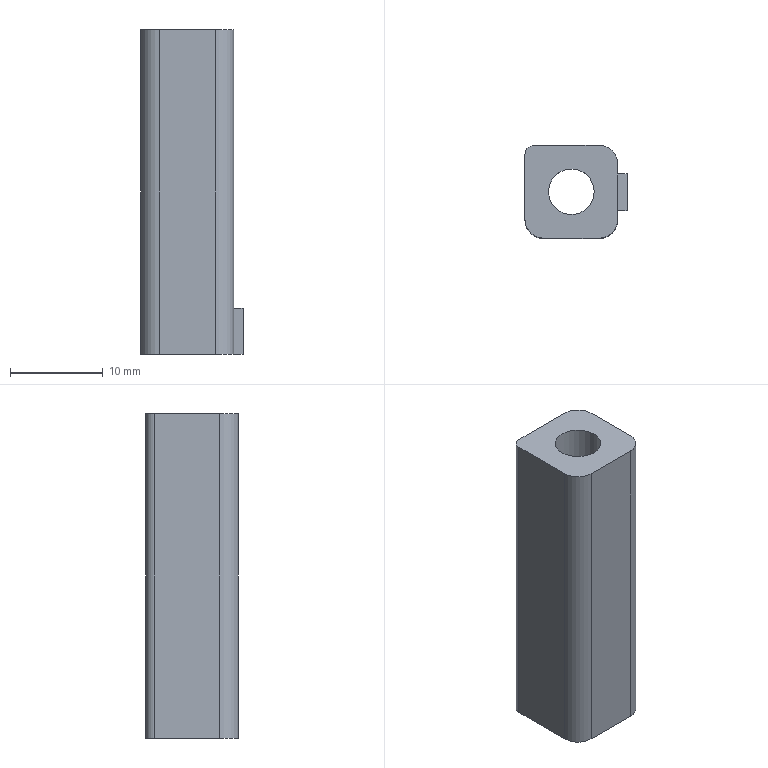Part | NX | features DIE-89 2 | 1 solid | 17 faces | box 11 x 10 x 35 mm | volume 2502 mm3 | plane 11 | cylinder 6 | commonest cylinder face diameters 4 x3 2 x1 4.92 x1 5.92 x1
STEP:
#1=CARTESIAN_POINT('',(4085.776,-839.123,858.716));
#2=VERTEX_POINT('',#1);
#3=CARTESIAN_POINT('',(4085.776,-839.123,853.716));
#4=VERTEX_POINT('',#3);
#5=CARTESIAN_POINT('',(4085.776,-839.123,862.216));
#6=DIRECTION('',(0.,0.,-1.));
#7=VECTOR('',#6,1000.);
#8=LINE('',#5,#7);
#9=EDGE_CURVE('',#2,#4,#8,.T.);
#10=ORIENTED_EDGE('',*,*,#9,.F.);
#11=CARTESIAN_POINT('',(4088.236,-839.123,858.716));
#12=DIRECTION('',(0.,0.,-1.));
#13=DIRECTION('',(1.,0.,0.));
#14=AXIS2_PLACEMENT_3D('',#11,#12,#13);
#15=CIRCLE('',#14,2.46);
#16=EDGE_CURVE('',#2,#2,#15,.T.);
#17=ORIENTED_EDGE('',*,*,#16,.F.);
#18=ORIENTED_EDGE('',*,*,#9,.T.);
#19=CARTESIAN_POINT('',(4088.236,-839.123,853.716));
#20=DIRECTION('',(0.,0.,-1.));
#21=DIRECTION('',(1.,0.,0.));
#22=AXIS2_PLACEMENT_3D('',#19,#20,#21);
#23=CIRCLE('',#22,2.46);
#24=EDGE_CURVE('',#4,#4,#23,.F.);
#25=ORIENTED_EDGE('',*,*,#24,.F.);
#26=EDGE_LOOP('',(#10,#17,#18,#25));
#27=FACE_BOUND('',#26,.T.);
#28=CARTESIAN_POINT('',(4088.236,-839.123,862.216));
#29=DIRECTION('',(0.,0.,-1.));
#30=DIRECTION('',(-1.,0.,0.));
#31=AXIS2_PLACEMENT_3D('',#28,#29,#30);
#32=CYLINDRICAL_SURFACE('',#31,2.46);
#33=ADVANCED_FACE('',(#27),#32,.F.);
#34=ORIENTED_EDGE('',*,*,#16,.T.);
#35=EDGE_LOOP('',(#34));
#36=FACE_BOUND('',#35,.T.);
#37=CARTESIAN_POINT('',(4083.236,-842.123,858.716));
#38=VERTEX_POINT('',#37);
#39=CARTESIAN_POINT('',(4083.236,-835.123,858.716));
#40=VERTEX_POINT('',#39);
#41=CARTESIAN_POINT('',(4083.236,-839.123,858.716));
#42=DIRECTION('',(0.,1.,0.));
#43=VECTOR('',#42,1000.);
#44=LINE('',#41,#43);
#45=EDGE_CURVE('',#38,#40,#44,.T.);
#46=ORIENTED_EDGE('',*,*,#45,.F.);
#47=CARTESIAN_POINT('',(4085.236,-844.123,858.716));
#48=VERTEX_POINT('',#47);
#49=CARTESIAN_POINT('',(4085.236,-842.123,858.716));
#50=DIRECTION('',(0.,0.,1.));
#51=DIRECTION('',(1.,0.,0.));
#52=AXIS2_PLACEMENT_3D('',#49,#50,#51);
#53=CIRCLE('',#52,2.);
#54=EDGE_CURVE('',#48,#38,#53,.F.);
#55=ORIENTED_EDGE('',*,*,#54,.F.);
#56=CARTESIAN_POINT('',(4091.236,-844.123,858.716));
#57=VERTEX_POINT('',#56);
#58=CARTESIAN_POINT('',(4088.236,-844.123,858.716));
#59=DIRECTION('',(-1.,0.,0.));
#60=VECTOR('',#59,1000.);
#61=LINE('',#58,#60);
#62=EDGE_CURVE('',#48,#57,#61,.F.);
#63=ORIENTED_EDGE('',*,*,#62,.T.);
#64=CARTESIAN_POINT('',(4093.236,-842.123,858.716));
#65=VERTEX_POINT('',#64);
#66=CARTESIAN_POINT('',(4091.236,-842.123,858.716));
#67=DIRECTION('',(0.,0.,1.));
#68=DIRECTION('',(1.,0.,0.));
#69=AXIS2_PLACEMENT_3D('',#66,#67,#68);
#70=CIRCLE('',#69,2.);
#71=EDGE_CURVE('',#65,#57,#70,.F.);
#72=ORIENTED_EDGE('',*,*,#71,.F.);
#73=CARTESIAN_POINT('',(4093.236,-836.123,858.716));
#74=VERTEX_POINT('',#73);
#75=CARTESIAN_POINT('',(4093.236,-839.123,858.716));
#76=DIRECTION('',(0.,-1.,0.));
#77=VECTOR('',#76,1000.);
#78=LINE('',#75,#77);
#79=EDGE_CURVE('',#65,#74,#78,.F.);
#80=ORIENTED_EDGE('',*,*,#79,.T.);
#81=CARTESIAN_POINT('',(4091.236,-834.123,858.716));
#82=VERTEX_POINT('',#81);
#83=CARTESIAN_POINT('',(4091.236,-836.123,858.716));
#84=DIRECTION('',(0.,0.,1.));
#85=DIRECTION('',(1.,0.,0.));
#86=AXIS2_PLACEMENT_3D('',#83,#84,#85);
#87=CIRCLE('',#86,2.);
#88=EDGE_CURVE('',#74,#82,#87,.T.);
#89=ORIENTED_EDGE('',*,*,#88,.T.);
#90=CARTESIAN_POINT('',(4084.236,-834.123,858.716));
#91=VERTEX_POINT('',#90);
#92=CARTESIAN_POINT('',(4088.236,-834.123,858.716));
#93=DIRECTION('',(1.,0.,0.));
#94=VECTOR('',#93,1000.);
#95=LINE('',#92,#94);
#96=EDGE_CURVE('',#91,#82,#95,.T.);
#97=ORIENTED_EDGE('',*,*,#96,.F.);
#98=CARTESIAN_POINT('',(4084.236,-835.123,858.716));
#99=DIRECTION('',(0.,0.,1.));
#100=DIRECTION('',(1.,0.,0.));
#101=AXIS2_PLACEMENT_3D('',#98,#99,#100);
#102=CIRCLE('',#101,1.);
#103=EDGE_CURVE('',#40,#91,#102,.F.);
#104=ORIENTED_EDGE('',*,*,#103,.F.);
#105=EDGE_LOOP('',(#46,#55,#63,#72,#80,#89,#97,#104));
#106=FACE_BOUND('',#105,.T.);
#107=CARTESIAN_POINT('',(4079.736,-858.123,858.716));
#108=DIRECTION('',(0.,0.,1.));
#109=DIRECTION('',(1.,0.,0.));
#110=AXIS2_PLACEMENT_3D('',#107,#108,#109);
#111=PLANE('',#110);
#112=ADVANCED_FACE('',(#36,#106),#111,.T.);
#113=CARTESIAN_POINT('',(4085.276,-839.123,853.716));
#114=VERTEX_POINT('',#113);
#115=CARTESIAN_POINT('',(4088.236,-839.123,853.716));
#116=DIRECTION('',(0.,0.,1.));
#117=DIRECTION('',(1.,0.,0.));
#118=AXIS2_PLACEMENT_3D('',#115,#116,#117);
#119=CIRCLE('',#118,2.96);
#120=EDGE_CURVE('',#114,#114,#119,.F.);
#121=ORIENTED_EDGE('',*,*,#120,.T.);
#122=EDGE_LOOP('',(#121));
#123=FACE_BOUND('',#122,.T.);
#124=ORIENTED_EDGE('',*,*,#24,.T.);
#125=EDGE_LOOP('',(#124));
#126=FACE_BOUND('',#125,.T.);
#127=CARTESIAN_POINT('',(4079.736,-858.123,853.716));
#128=DIRECTION('',(0.,0.,1.));
#129=DIRECTION('',(1.,0.,0.));
#130=AXIS2_PLACEMENT_3D('',#127,#128,#129);
#131=PLANE('',#130);
#132=ADVANCED_FACE('',(#123,#126),#131,.F.);
#133=CARTESIAN_POINT('',(4085.276,-839.123,823.716));
#134=VERTEX_POINT('',#133);
#135=CARTESIAN_POINT('',(4088.236,-839.123,823.716));
#136=DIRECTION('',(0.,0.,-1.));
#137=DIRECTION('',(-1.,0.,0.));
#138=AXIS2_PLACEMENT_3D('',#135,#136,#137);
#139=CIRCLE('',#138,2.96);
#140=EDGE_CURVE('',#134,#134,#139,.T.);
#141=ORIENTED_EDGE('',*,*,#140,.T.);
#142=CARTESIAN_POINT('',(4085.276,-839.123,862.216));
#143=DIRECTION('',(0.,0.,-1.));
#144=VECTOR('',#143,1000.);
#145=LINE('',#142,#144);
#146=EDGE_CURVE('',#114,#134,#145,.T.);
#147=ORIENTED_EDGE('',*,*,#146,.F.);
#148=ORIENTED_EDGE('',*,*,#120,.F.);
#149=ORIENTED_EDGE('',*,*,#146,.T.);
#150=EDGE_LOOP('',(#141,#147,#148,#149));
#151=FACE_BOUND('',#150,.T.);
#152=CARTESIAN_POINT('',(4088.236,-839.123,862.216));
#153=DIRECTION('',(0.,0.,-1.));
#154=DIRECTION('',(-1.,0.,0.));
#155=AXIS2_PLACEMENT_3D('',#152,#153,#154);
#156=CYLINDRICAL_SURFACE('',#155,2.96);
#157=ADVANCED_FACE('',(#151),#156,.F.);
#158=CARTESIAN_POINT('',(4093.236,-837.123,823.716));
#159=VERTEX_POINT('',#158);
#160=CARTESIAN_POINT('',(4093.236,-836.123,823.716));
#161=VERTEX_POINT('',#160);
#162=CARTESIAN_POINT('',(4093.236,-839.123,823.716));
#163=DIRECTION('',(0.,1.,0.));
#164=VECTOR('',#163,1000.);
#165=LINE('',#162,#164);
#166=EDGE_CURVE('',#159,#161,#165,.T.);
#167=ORIENTED_EDGE('',*,*,#166,.F.);
#168=CARTESIAN_POINT('',(4094.236,-837.123,823.716));
#169=VERTEX_POINT('',#168);
#170=CARTESIAN_POINT('',(0.,-837.123,823.716));
#171=DIRECTION('',(1.,0.,0.));
#172=VECTOR('',#171,1000.);
#173=LINE('',#170,#172);
#174=EDGE_CURVE('',#159,#169,#173,.T.);
#175=ORIENTED_EDGE('',*,*,#174,.T.);
#176=CARTESIAN_POINT('',(4094.236,-841.123,823.716));
#177=VERTEX_POINT('',#176);
#178=CARTESIAN_POINT('',(4094.236,-836.123,823.716));
#179=DIRECTION('',(0.,-1.,0.));
#180=VECTOR('',#179,1000.);
#181=LINE('',#178,#180);
#182=EDGE_CURVE('',#169,#177,#181,.T.);
#183=ORIENTED_EDGE('',*,*,#182,.T.);
#184=CARTESIAN_POINT('',(4093.236,-841.123,823.716));
#185=VERTEX_POINT('',#184);
#186=CARTESIAN_POINT('',(0.,-841.123,823.716));
#187=DIRECTION('',(-1.,0.,0.));
#188=VECTOR('',#187,1000.);
#189=LINE('',#186,#188);
#190=EDGE_CURVE('',#177,#185,#189,.T.);
#191=ORIENTED_EDGE('',*,*,#190,.T.);
#192=CARTESIAN_POINT('',(4093.236,-842.123,823.716));
#193=VERTEX_POINT('',#192);
#194=CARTESIAN_POINT('',(4093.236,-839.123,823.716));
#195=DIRECTION('',(0.,1.,0.));
#196=VECTOR('',#195,1000.);
#197=LINE('',#194,#196);
#198=EDGE_CURVE('',#193,#185,#197,.T.);
#199=ORIENTED_EDGE('',*,*,#198,.F.);
#200=CARTESIAN_POINT('',(4091.236,-844.123,823.716));
#201=VERTEX_POINT('',#200);
#202=CARTESIAN_POINT('',(4091.236,-842.123,823.716));
#203=DIRECTION('',(0.,0.,-1.));
#204=DIRECTION('',(-1.,0.,0.));
#205=AXIS2_PLACEMENT_3D('',#202,#203,#204);
#206=CIRCLE('',#205,2.);
#207=EDGE_CURVE('',#193,#201,#206,.T.);
#208=ORIENTED_EDGE('',*,*,#207,.T.);
#209=CARTESIAN_POINT('',(4085.236,-844.123,823.716));
#210=VERTEX_POINT('',#209);
#211=CARTESIAN_POINT('',(4088.236,-844.123,823.716));
#212=DIRECTION('',(1.,0.,0.));
#213=VECTOR('',#212,1000.);
#214=LINE('',#211,#213);
#215=EDGE_CURVE('',#210,#201,#214,.T.);
#216=ORIENTED_EDGE('',*,*,#215,.F.);
#217=CARTESIAN_POINT('',(4083.236,-842.123,823.716));
#218=VERTEX_POINT('',#217);
#219=CARTESIAN_POINT('',(4085.236,-842.123,823.716));
#220=DIRECTION('',(0.,0.,-1.));
#221=DIRECTION('',(-1.,0.,0.));
#222=AXIS2_PLACEMENT_3D('',#219,#220,#221);
#223=CIRCLE('',#222,2.);
#224=EDGE_CURVE('',#218,#210,#223,.F.);
#225=ORIENTED_EDGE('',*,*,#224,.F.);
#226=CARTESIAN_POINT('',(4083.236,-835.123,823.716));
#227=VERTEX_POINT('',#226);
#228=CARTESIAN_POINT('',(4083.236,-839.123,823.716));
#229=DIRECTION('',(0.,-1.,0.));
#230=VECTOR('',#229,1000.);
#231=LINE('',#228,#230);
#232=EDGE_CURVE('',#227,#218,#231,.T.);
#233=ORIENTED_EDGE('',*,*,#232,.F.);
#234=CARTESIAN_POINT('',(4084.236,-834.123,823.716));
#235=VERTEX_POINT('',#234);
#236=CARTESIAN_POINT('',(4084.236,-835.123,823.716));
#237=DIRECTION('',(0.,0.,-1.));
#238=DIRECTION('',(-1.,0.,0.));
#239=AXIS2_PLACEMENT_3D('',#236,#237,#238);
#240=CIRCLE('',#239,1.);
#241=EDGE_CURVE('',#227,#235,#240,.T.);
#242=ORIENTED_EDGE('',*,*,#241,.T.);
#243=CARTESIAN_POINT('',(4091.236,-834.123,823.716));
#244=VERTEX_POINT('',#243);
#245=CARTESIAN_POINT('',(4088.236,-834.123,823.716));
#246=DIRECTION('',(-1.,0.,0.));
#247=VECTOR('',#246,1000.);
#248=LINE('',#245,#247);
#249=EDGE_CURVE('',#244,#235,#248,.T.);
#250=ORIENTED_EDGE('',*,*,#249,.F.);
#251=CARTESIAN_POINT('',(4091.236,-836.123,823.716));
#252=DIRECTION('',(0.,0.,-1.));
#253=DIRECTION('',(-1.,0.,0.));
#254=AXIS2_PLACEMENT_3D('',#251,#252,#253);
#255=CIRCLE('',#254,2.);
#256=EDGE_CURVE('',#161,#244,#255,.F.);
#257=ORIENTED_EDGE('',*,*,#256,.F.);
#258=EDGE_LOOP('',(#167,#175,#183,#191,#199,#208,#216,#225,#233,#242,#250,#257));
#259=FACE_BOUND('',#258,.T.);
#260=ORIENTED_EDGE('',*,*,#140,.F.);
#261=EDGE_LOOP('',(#260));
#262=FACE_BOUND('',#261,.T.);
#263=CARTESIAN_POINT('',(4123.586,-858.123,823.716));
#264=DIRECTION('',(0.,0.,-1.));
#265=DIRECTION('',(-1.,0.,0.));
#266=AXIS2_PLACEMENT_3D('',#263,#264,#265);
#267=PLANE('',#266);
#268=ADVANCED_FACE('',(#259,#262),#267,.T.);
#269=ORIENTED_EDGE('',*,*,#241,.F.);
#270=CARTESIAN_POINT('',(4083.236,-835.123,823.716));
#271=DIRECTION('',(0.,0.,1.));
#272=VECTOR('',#271,1000.);
#273=LINE('',#270,#272);
#274=EDGE_CURVE('',#40,#227,#273,.F.);
#275=ORIENTED_EDGE('',*,*,#274,.F.);
#276=ORIENTED_EDGE('',*,*,#103,.T.);
#277=CARTESIAN_POINT('',(4084.236,-834.123,823.716));
#278=DIRECTION('',(0.,0.,1.));
#279=VECTOR('',#278,1000.);
#280=LINE('',#277,#279);
#281=EDGE_CURVE('',#235,#91,#280,.T.);
#282=ORIENTED_EDGE('',*,*,#281,.F.);
#283=EDGE_LOOP('',(#269,#275,#276,#282));
#284=FACE_BOUND('',#283,.T.);
#285=CARTESIAN_POINT('',(4084.236,-835.123,823.716));
#286=DIRECTION('',(0.,0.,1.));
#287=DIRECTION('',(1.,0.,0.));
#288=AXIS2_PLACEMENT_3D('',#285,#286,#287);
#289=CYLINDRICAL_SURFACE('',#288,1.);
#290=ADVANCED_FACE('',(#284),#289,.T.);
#291=ORIENTED_EDGE('',*,*,#224,.T.);
#292=CARTESIAN_POINT('',(4085.236,-844.123,823.716));
#293=DIRECTION('',(0.,0.,1.));
#294=VECTOR('',#293,1000.);
#295=LINE('',#292,#294);
#296=EDGE_CURVE('',#48,#210,#295,.F.);
#297=ORIENTED_EDGE('',*,*,#296,.F.);
#298=ORIENTED_EDGE('',*,*,#54,.T.);
#299=CARTESIAN_POINT('',(4083.236,-842.123,823.716));
#300=DIRECTION('',(0.,0.,1.));
#301=VECTOR('',#300,1000.);
#302=LINE('',#299,#301);
#303=EDGE_CURVE('',#218,#38,#302,.T.);
#304=ORIENTED_EDGE('',*,*,#303,.F.);
#305=EDGE_LOOP('',(#291,#297,#298,#304));
#306=FACE_BOUND('',#305,.T.);
#307=CARTESIAN_POINT('',(4085.236,-842.123,823.716));
#308=DIRECTION('',(0.,0.,1.));
#309=DIRECTION('',(1.,0.,0.));
#310=AXIS2_PLACEMENT_3D('',#307,#308,#309);
#311=CYLINDRICAL_SURFACE('',#310,2.);
#312=ADVANCED_FACE('',(#306),#311,.T.);
#313=ORIENTED_EDGE('',*,*,#207,.F.);
#314=CARTESIAN_POINT('',(4093.236,-842.123,823.716));
#315=DIRECTION('',(0.,0.,1.));
#316=VECTOR('',#315,1000.);
#317=LINE('',#314,#316);
#318=EDGE_CURVE('',#65,#193,#317,.F.);
#319=ORIENTED_EDGE('',*,*,#318,.F.);
#320=ORIENTED_EDGE('',*,*,#71,.T.);
#321=CARTESIAN_POINT('',(4091.236,-844.123,823.716));
#322=DIRECTION('',(0.,0.,1.));
#323=VECTOR('',#322,1000.);
#324=LINE('',#321,#323);
#325=EDGE_CURVE('',#201,#57,#324,.T.);
#326=ORIENTED_EDGE('',*,*,#325,.F.);
#327=EDGE_LOOP('',(#313,#319,#320,#326));
#328=FACE_BOUND('',#327,.T.);
#329=CARTESIAN_POINT('',(4091.236,-842.123,823.716));
#330=DIRECTION('',(0.,0.,1.));
#331=DIRECTION('',(1.,0.,0.));
#332=AXIS2_PLACEMENT_3D('',#329,#330,#331);
#333=CYLINDRICAL_SURFACE('',#332,2.);
#334=ADVANCED_FACE('',(#328),#333,.T.);
#335=ORIENTED_EDGE('',*,*,#256,.T.);
#336=CARTESIAN_POINT('',(4091.236,-834.123,823.716));
#337=DIRECTION('',(0.,0.,1.));
#338=VECTOR('',#337,1000.);
#339=LINE('',#336,#338);
#340=EDGE_CURVE('',#82,#244,#339,.F.);
#341=ORIENTED_EDGE('',*,*,#340,.F.);
#342=ORIENTED_EDGE('',*,*,#88,.F.);
#343=CARTESIAN_POINT('',(4093.236,-836.123,823.716));
#344=DIRECTION('',(0.,0.,1.));
#345=VECTOR('',#344,1000.);
#346=LINE('',#343,#345);
#347=EDGE_CURVE('',#161,#74,#346,.T.);
#348=ORIENTED_EDGE('',*,*,#347,.F.);
#349=EDGE_LOOP('',(#335,#341,#342,#348));
#350=FACE_BOUND('',#349,.T.);
#351=CARTESIAN_POINT('',(4091.236,-836.123,823.716));
#352=DIRECTION('',(0.,0.,1.));
#353=DIRECTION('',(1.,0.,0.));
#354=AXIS2_PLACEMENT_3D('',#351,#352,#353);
#355=CYLINDRICAL_SURFACE('',#354,2.);
#356=ADVANCED_FACE('',(#350),#355,.T.);
#357=CARTESIAN_POINT('',(4093.236,-841.123,828.716));
#358=VERTEX_POINT('',#357);
#359=CARTESIAN_POINT('',(4093.236,-841.123,823.716));
#360=DIRECTION('',(0.,0.,-1.));
#361=VECTOR('',#360,1000.);
#362=LINE('',#359,#361);
#363=EDGE_CURVE('',#358,#185,#362,.T.);
#364=ORIENTED_EDGE('',*,*,#363,.F.);
#365=CARTESIAN_POINT('',(4093.236,-837.123,828.716));
#366=VERTEX_POINT('',#365);
#367=CARTESIAN_POINT('',(4093.236,-839.123,828.716));
#368=DIRECTION('',(0.,1.,0.));
#369=VECTOR('',#368,1000.);
#370=LINE('',#367,#369);
#371=EDGE_CURVE('',#358,#366,#370,.T.);
#372=ORIENTED_EDGE('',*,*,#371,.T.);
#373=CARTESIAN_POINT('',(4093.236,-837.123,823.716));
#374=DIRECTION('',(0.,0.,1.));
#375=VECTOR('',#374,1000.);
#376=LINE('',#373,#375);
#377=EDGE_CURVE('',#159,#366,#376,.T.);
#378=ORIENTED_EDGE('',*,*,#377,.F.);
#379=ORIENTED_EDGE('',*,*,#166,.T.);
#380=ORIENTED_EDGE('',*,*,#347,.T.);
#381=ORIENTED_EDGE('',*,*,#79,.F.);
#382=ORIENTED_EDGE('',*,*,#318,.T.);
#383=ORIENTED_EDGE('',*,*,#198,.T.);
#384=EDGE_LOOP('',(#364,#372,#378,#379,#380,#381,#382,#383));
#385=FACE_BOUND('',#384,.T.);
#386=CARTESIAN_POINT('',(4093.236,-839.123,823.716));
#387=DIRECTION('',(1.,0.,0.));
#388=DIRECTION('',(0.,0.,-1.));
#389=AXIS2_PLACEMENT_3D('',#386,#387,#388);
#390=PLANE('',#389);
#391=ADVANCED_FACE('',(#385),#390,.T.);
#392=ORIENTED_EDGE('',*,*,#249,.T.);
#393=ORIENTED_EDGE('',*,*,#281,.T.);
#394=ORIENTED_EDGE('',*,*,#96,.T.);
#395=ORIENTED_EDGE('',*,*,#340,.T.);
#396=EDGE_LOOP('',(#392,#393,#394,#395));
#397=FACE_BOUND('',#396,.T.);
#398=CARTESIAN_POINT('',(4088.236,-834.123,823.716));
#399=DIRECTION('',(0.,1.,0.));
#400=DIRECTION('',(0.,0.,1.));
#401=AXIS2_PLACEMENT_3D('',#398,#399,#400);
#402=PLANE('',#401);
#403=ADVANCED_FACE('',(#397),#402,.T.);
#404=ORIENTED_EDGE('',*,*,#45,.T.);
#405=ORIENTED_EDGE('',*,*,#274,.T.);
#406=ORIENTED_EDGE('',*,*,#232,.T.);
#407=ORIENTED_EDGE('',*,*,#303,.T.);
#408=EDGE_LOOP('',(#404,#405,#406,#407));
#409=FACE_BOUND('',#408,.T.);
#410=CARTESIAN_POINT('',(4083.236,-839.123,823.716));
#411=DIRECTION('',(-1.,0.,0.));
#412=DIRECTION('',(0.,0.,1.));
#413=AXIS2_PLACEMENT_3D('',#410,#411,#412);
#414=PLANE('',#413);
#415=ADVANCED_FACE('',(#409),#414,.T.);
#416=ORIENTED_EDGE('',*,*,#215,.T.);
#417=ORIENTED_EDGE('',*,*,#325,.T.);
#418=ORIENTED_EDGE('',*,*,#62,.F.);
#419=ORIENTED_EDGE('',*,*,#296,.T.);
#420=EDGE_LOOP('',(#416,#417,#418,#419));
#421=FACE_BOUND('',#420,.T.);
#422=CARTESIAN_POINT('',(4088.236,-844.123,823.716));
#423=DIRECTION('',(0.,-1.,0.));
#424=DIRECTION('',(0.,0.,-1.));
#425=AXIS2_PLACEMENT_3D('',#422,#423,#424);
#426=PLANE('',#425);
#427=ADVANCED_FACE('',(#421),#426,.T.);
#428=CARTESIAN_POINT('',(4094.236,-841.123,828.716));
#429=VERTEX_POINT('',#428);
#430=CARTESIAN_POINT('',(0.,-841.123,828.716));
#431=DIRECTION('',(-1.,0.,0.));
#432=VECTOR('',#431,1000.);
#433=LINE('',#430,#432);
#434=EDGE_CURVE('',#429,#358,#433,.T.);
#435=ORIENTED_EDGE('',*,*,#434,.T.);
#436=ORIENTED_EDGE('',*,*,#363,.T.);
#437=ORIENTED_EDGE('',*,*,#190,.F.);
#438=CARTESIAN_POINT('',(4094.236,-841.123,828.716));
#439=DIRECTION('',(0.,0.,-1.));
#440=VECTOR('',#439,1000.);
#441=LINE('',#438,#440);
#442=EDGE_CURVE('',#429,#177,#441,.T.);
#443=ORIENTED_EDGE('',*,*,#442,.F.);
#444=EDGE_LOOP('',(#435,#436,#437,#443));
#445=FACE_BOUND('',#444,.T.);
#446=CARTESIAN_POINT('',(4094.236,-841.123,828.716));
#447=DIRECTION('',(0.,-1.,0.));
#448=DIRECTION('',(0.,0.,-1.));
#449=AXIS2_PLACEMENT_3D('',#446,#447,#448);
#450=PLANE('',#449);
#451=ADVANCED_FACE('',(#445),#450,.T.);
#452=ORIENTED_EDGE('',*,*,#174,.F.);
#453=ORIENTED_EDGE('',*,*,#377,.T.);
#454=CARTESIAN_POINT('',(4094.236,-837.123,828.716));
#455=VERTEX_POINT('',#454);
#456=CARTESIAN_POINT('',(0.,-837.123,828.716));
#457=DIRECTION('',(1.,0.,0.));
#458=VECTOR('',#457,1000.);
#459=LINE('',#456,#458);
#460=EDGE_CURVE('',#366,#455,#459,.T.);
#461=ORIENTED_EDGE('',*,*,#460,.T.);
#462=CARTESIAN_POINT('',(4094.236,-837.123,828.716));
#463=DIRECTION('',(0.,0.,-1.));
#464=VECTOR('',#463,1000.);
#465=LINE('',#462,#464);
#466=EDGE_CURVE('',#455,#169,#465,.T.);
#467=ORIENTED_EDGE('',*,*,#466,.T.);
#468=EDGE_LOOP('',(#452,#453,#461,#467));
#469=FACE_BOUND('',#468,.T.);
#470=CARTESIAN_POINT('',(4093.186,-837.123,828.716));
#471=DIRECTION('',(0.,1.,0.));
#472=DIRECTION('',(0.,0.,1.));
#473=AXIS2_PLACEMENT_3D('',#470,#471,#472);
#474=PLANE('',#473);
#475=ADVANCED_FACE('',(#469),#474,.T.);
#476=ORIENTED_EDGE('',*,*,#182,.F.);
#477=ORIENTED_EDGE('',*,*,#466,.F.);
#478=CARTESIAN_POINT('',(4094.236,-836.123,828.716));
#479=DIRECTION('',(0.,-1.,0.));
#480=VECTOR('',#479,1000.);
#481=LINE('',#478,#480);
#482=EDGE_CURVE('',#455,#429,#481,.T.);
#483=ORIENTED_EDGE('',*,*,#482,.T.);
#484=ORIENTED_EDGE('',*,*,#442,.T.);
#485=EDGE_LOOP('',(#476,#477,#483,#484));
#486=FACE_BOUND('',#485,.T.);
#487=CARTESIAN_POINT('',(4094.236,-836.123,828.716));
#488=DIRECTION('',(1.,0.,0.));
#489=DIRECTION('',(0.,0.,-1.));
#490=AXIS2_PLACEMENT_3D('',#487,#488,#489);
#491=PLANE('',#490);
#492=ADVANCED_FACE('',(#486),#491,.T.);
#493=ORIENTED_EDGE('',*,*,#371,.F.);
#494=ORIENTED_EDGE('',*,*,#434,.F.);
#495=ORIENTED_EDGE('',*,*,#482,.F.);
#496=ORIENTED_EDGE('',*,*,#460,.F.);
#497=EDGE_LOOP('',(#493,#494,#495,#496));
#498=FACE_BOUND('',#497,.T.);
#499=CARTESIAN_POINT('',(0.,0.,828.716));
#500=DIRECTION('',(0.,0.,-1.));
#501=DIRECTION('',(-1.,0.,0.));
#502=AXIS2_PLACEMENT_3D('',#499,#500,#501);
#503=PLANE('',#502);
#504=ADVANCED_FACE('',(#498),#503,.F.);
#505=CLOSED_SHELL('',(#33,#112,#132,#157,#268,#290,#312,#334,#356,#391,#403,#415,#427,#451,#475,#492,#504));
#506=MANIFOLD_SOLID_BREP('',#505);
#507=(LENGTH_UNIT()NAMED_UNIT(*)SI_UNIT(.MILLI.,.METRE.));
#508=UNCERTAINTY_MEASURE_WITH_UNIT(LENGTH_MEASURE(0.00001),#507,'','');
#509=(NAMED_UNIT(*)PLANE_ANGLE_UNIT()SI_UNIT($,.RADIAN.));
#510=(NAMED_UNIT(*)SI_UNIT($,.STERADIAN.)SOLID_ANGLE_UNIT());
#511=(GEOMETRIC_REPRESENTATION_CONTEXT(3)GLOBAL_UNCERTAINTY_ASSIGNED_CONTEXT((#508))GLOBAL_UNIT_ASSIGNED_CONTEXT((#507,#509,#510))REPRESENTATION_CONTEXT('',''));
#512=ADVANCED_BREP_SHAPE_REPRESENTATION('',(#506),#511);